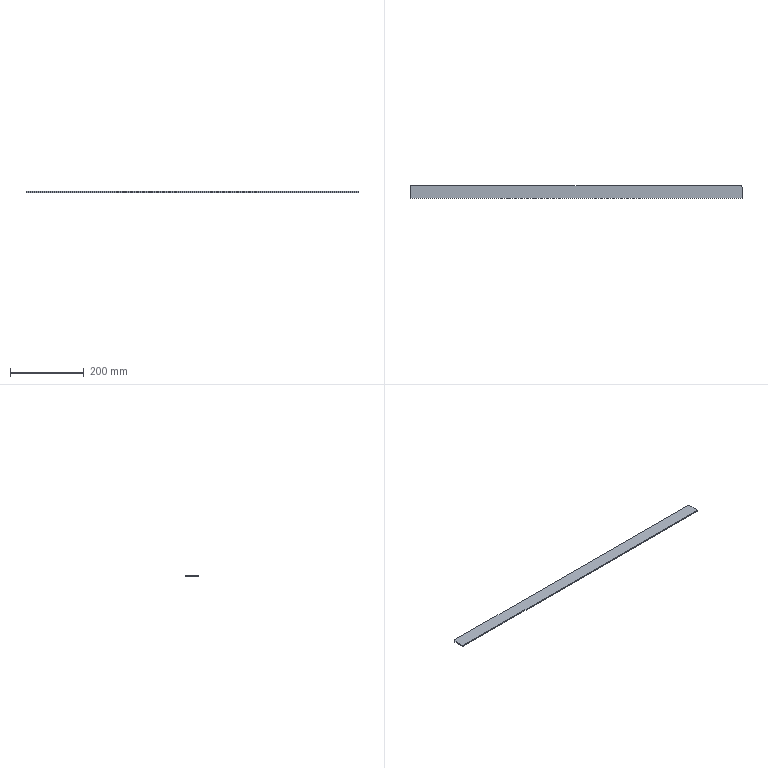Part | SolidWorks | features Extrusion 1, Fillet 1 | 1 solid | 8 faces | box 900 x 35 x 3 mm | volume 94468 mm3 | plane 6 | cylinder 2 | commonest cylinder face diameters 10 x2
STEP:
#1=CARTESIAN_POINT('',(450.,-17.5,0.));
#2=VERTEX_POINT('',#1);
#3=CARTESIAN_POINT('',(450.,12.5,0.));
#4=VERTEX_POINT('',#3);
#5=CARTESIAN_POINT('',(450.,17.5,0.));
#6=DIRECTION('',(0.,1.,0.));
#7=VECTOR('',#6,1000.);
#8=LINE('',#5,#7);
#9=EDGE_CURVE('',#2,#4,#8,.T.);
#10=ORIENTED_EDGE('',*,*,#9,.T.);
#11=CARTESIAN_POINT('',(450.,12.5,3.));
#12=VERTEX_POINT('',#11);
#13=CARTESIAN_POINT('',(450.,12.5,3.));
#14=DIRECTION('',(0.,0.,1.));
#15=VECTOR('',#14,1000.);
#16=LINE('',#13,#15);
#17=EDGE_CURVE('',#4,#12,#16,.T.);
#18=ORIENTED_EDGE('',*,*,#17,.T.);
#19=CARTESIAN_POINT('',(450.,-17.5,3.));
#20=VERTEX_POINT('',#19);
#21=CARTESIAN_POINT('',(450.,17.5,3.));
#22=DIRECTION('',(0.,1.,0.));
#23=VECTOR('',#22,1000.);
#24=LINE('',#21,#23);
#25=EDGE_CURVE('',#20,#12,#24,.T.);
#26=ORIENTED_EDGE('',*,*,#25,.F.);
#27=CARTESIAN_POINT('',(450.,-17.5,3.));
#28=DIRECTION('',(0.,0.,-1.));
#29=VECTOR('',#28,1000.);
#30=LINE('',#27,#29);
#31=EDGE_CURVE('',#20,#2,#30,.T.);
#32=ORIENTED_EDGE('',*,*,#31,.T.);
#33=EDGE_LOOP('',(#10,#18,#26,#32));
#34=FACE_OUTER_BOUND('',#33,.T.);
#35=CARTESIAN_POINT('',(450.,17.5,3.));
#36=DIRECTION('',(-1.,0.,0.));
#37=DIRECTION('',(0.,0.,1.));
#38=AXIS2_PLACEMENT_3D('',#35,#36,#37);
#39=PLANE('',#38);
#40=ADVANCED_FACE('',(#34),#39,.F.);
#41=CARTESIAN_POINT('',(445.,17.5,0.));
#42=VERTEX_POINT('',#41);
#43=CARTESIAN_POINT('',(-445.,17.5,0.));
#44=VERTEX_POINT('',#43);
#45=CARTESIAN_POINT('',(-450.,17.5,0.));
#46=DIRECTION('',(-1.,0.,0.));
#47=VECTOR('',#46,1000.);
#48=LINE('',#45,#47);
#49=EDGE_CURVE('',#42,#44,#48,.T.);
#50=ORIENTED_EDGE('',*,*,#49,.T.);
#51=CARTESIAN_POINT('',(-445.,17.5,3.));
#52=VERTEX_POINT('',#51);
#53=CARTESIAN_POINT('',(-445.,17.5,3.));
#54=DIRECTION('',(0.,0.,1.));
#55=VECTOR('',#54,1000.);
#56=LINE('',#53,#55);
#57=EDGE_CURVE('',#44,#52,#56,.T.);
#58=ORIENTED_EDGE('',*,*,#57,.T.);
#59=CARTESIAN_POINT('',(445.,17.5,3.));
#60=VERTEX_POINT('',#59);
#61=CARTESIAN_POINT('',(-450.,17.5,3.));
#62=DIRECTION('',(-1.,0.,0.));
#63=VECTOR('',#62,1000.);
#64=LINE('',#61,#63);
#65=EDGE_CURVE('',#60,#52,#64,.T.);
#66=ORIENTED_EDGE('',*,*,#65,.F.);
#67=CARTESIAN_POINT('',(445.,17.5,3.));
#68=DIRECTION('',(0.,0.,-1.));
#69=VECTOR('',#68,1000.);
#70=LINE('',#67,#69);
#71=EDGE_CURVE('',#60,#42,#70,.T.);
#72=ORIENTED_EDGE('',*,*,#71,.T.);
#73=EDGE_LOOP('',(#50,#58,#66,#72));
#74=FACE_OUTER_BOUND('',#73,.T.);
#75=CARTESIAN_POINT('',(-450.,17.5,3.));
#76=DIRECTION('',(0.,-1.,0.));
#77=DIRECTION('',(0.,0.,-1.));
#78=AXIS2_PLACEMENT_3D('',#75,#76,#77);
#79=PLANE('',#78);
#80=ADVANCED_FACE('',(#74),#79,.F.);
#81=CARTESIAN_POINT('',(-450.,12.5,3.));
#82=VERTEX_POINT('',#81);
#83=CARTESIAN_POINT('',(-450.,-17.5,3.));
#84=VERTEX_POINT('',#83);
#85=CARTESIAN_POINT('',(-450.,17.5,3.));
#86=DIRECTION('',(0.,-1.,0.));
#87=VECTOR('',#86,1000.);
#88=LINE('',#85,#87);
#89=EDGE_CURVE('',#82,#84,#88,.T.);
#90=ORIENTED_EDGE('',*,*,#89,.F.);
#91=CARTESIAN_POINT('',(-450.,12.5,0.));
#92=VERTEX_POINT('',#91);
#93=CARTESIAN_POINT('',(-450.,12.5,3.));
#94=DIRECTION('',(0.,0.,-1.));
#95=VECTOR('',#94,1000.);
#96=LINE('',#93,#95);
#97=EDGE_CURVE('',#82,#92,#96,.T.);
#98=ORIENTED_EDGE('',*,*,#97,.T.);
#99=CARTESIAN_POINT('',(-450.,-17.5,0.));
#100=VERTEX_POINT('',#99);
#101=CARTESIAN_POINT('',(-450.,17.5,0.));
#102=DIRECTION('',(0.,-1.,0.));
#103=VECTOR('',#102,1000.);
#104=LINE('',#101,#103);
#105=EDGE_CURVE('',#92,#100,#104,.T.);
#106=ORIENTED_EDGE('',*,*,#105,.T.);
#107=CARTESIAN_POINT('',(-450.,-17.5,3.));
#108=DIRECTION('',(0.,0.,-1.));
#109=VECTOR('',#108,1000.);
#110=LINE('',#107,#109);
#111=EDGE_CURVE('',#84,#100,#110,.T.);
#112=ORIENTED_EDGE('',*,*,#111,.F.);
#113=EDGE_LOOP('',(#90,#98,#106,#112));
#114=FACE_OUTER_BOUND('',#113,.T.);
#115=CARTESIAN_POINT('',(-450.,17.5,3.));
#116=DIRECTION('',(1.,0.,0.));
#117=DIRECTION('',(0.,0.,-1.));
#118=AXIS2_PLACEMENT_3D('',#115,#116,#117);
#119=PLANE('',#118);
#120=ADVANCED_FACE('',(#114),#119,.F.);
#121=CARTESIAN_POINT('',(-450.,-17.5,0.));
#122=DIRECTION('',(1.,0.,0.));
#123=VECTOR('',#122,1000.);
#124=LINE('',#121,#123);
#125=EDGE_CURVE('',#100,#2,#124,.T.);
#126=ORIENTED_EDGE('',*,*,#125,.T.);
#127=ORIENTED_EDGE('',*,*,#31,.F.);
#128=CARTESIAN_POINT('',(-450.,-17.5,3.));
#129=DIRECTION('',(1.,0.,0.));
#130=VECTOR('',#129,1000.);
#131=LINE('',#128,#130);
#132=EDGE_CURVE('',#84,#20,#131,.T.);
#133=ORIENTED_EDGE('',*,*,#132,.F.);
#134=ORIENTED_EDGE('',*,*,#111,.T.);
#135=EDGE_LOOP('',(#126,#127,#133,#134));
#136=FACE_OUTER_BOUND('',#135,.T.);
#137=CARTESIAN_POINT('',(-450.,-17.5,3.));
#138=DIRECTION('',(0.,1.,0.));
#139=DIRECTION('',(0.,0.,1.));
#140=AXIS2_PLACEMENT_3D('',#137,#138,#139);
#141=PLANE('',#140);
#142=ADVANCED_FACE('',(#136),#141,.F.);
#143=ORIENTED_EDGE('',*,*,#65,.T.);
#144=CARTESIAN_POINT('',(-445.,12.5,3.));
#145=DIRECTION('',(0.,0.,1.));
#146=DIRECTION('',(1.,0.,0.));
#147=AXIS2_PLACEMENT_3D('',#144,#145,#146);
#148=CIRCLE('',#147,5.);
#149=EDGE_CURVE('',#52,#82,#148,.T.);
#150=ORIENTED_EDGE('',*,*,#149,.T.);
#151=ORIENTED_EDGE('',*,*,#89,.T.);
#152=ORIENTED_EDGE('',*,*,#132,.T.);
#153=ORIENTED_EDGE('',*,*,#25,.T.);
#154=CARTESIAN_POINT('',(445.,12.5,3.));
#155=DIRECTION('',(0.,0.,1.));
#156=DIRECTION('',(1.,0.,0.));
#157=AXIS2_PLACEMENT_3D('',#154,#155,#156);
#158=CIRCLE('',#157,5.);
#159=EDGE_CURVE('',#12,#60,#158,.T.);
#160=ORIENTED_EDGE('',*,*,#159,.T.);
#161=EDGE_LOOP('',(#143,#150,#151,#152,#153,#160));
#162=FACE_OUTER_BOUND('',#161,.T.);
#163=CARTESIAN_POINT('',(0.,0.,3.));
#164=DIRECTION('',(0.,0.,1.));
#165=DIRECTION('',(1.,0.,0.));
#166=AXIS2_PLACEMENT_3D('',#163,#164,#165);
#167=PLANE('',#166);
#168=ADVANCED_FACE('',(#162),#167,.T.);
#169=ORIENTED_EDGE('',*,*,#105,.F.);
#170=CARTESIAN_POINT('',(-445.,12.5,0.));
#171=DIRECTION('',(0.,0.,-1.));
#172=DIRECTION('',(1.,0.,0.));
#173=AXIS2_PLACEMENT_3D('',#170,#171,#172);
#174=CIRCLE('',#173,5.);
#175=EDGE_CURVE('',#92,#44,#174,.T.);
#176=ORIENTED_EDGE('',*,*,#175,.T.);
#177=ORIENTED_EDGE('',*,*,#49,.F.);
#178=CARTESIAN_POINT('',(445.,12.5,0.));
#179=DIRECTION('',(0.,0.,-1.));
#180=DIRECTION('',(1.,0.,0.));
#181=AXIS2_PLACEMENT_3D('',#178,#179,#180);
#182=CIRCLE('',#181,5.);
#183=EDGE_CURVE('',#42,#4,#182,.T.);
#184=ORIENTED_EDGE('',*,*,#183,.T.);
#185=ORIENTED_EDGE('',*,*,#9,.F.);
#186=ORIENTED_EDGE('',*,*,#125,.F.);
#187=EDGE_LOOP('',(#169,#176,#177,#184,#185,#186));
#188=FACE_OUTER_BOUND('',#187,.T.);
#189=CARTESIAN_POINT('',(0.,0.,0.));
#190=DIRECTION('',(0.,0.,1.));
#191=DIRECTION('',(1.,0.,0.));
#192=AXIS2_PLACEMENT_3D('',#189,#190,#191);
#193=PLANE('',#192);
#194=ADVANCED_FACE('',(#188),#193,.F.);
#195=ORIENTED_EDGE('',*,*,#149,.F.);
#196=ORIENTED_EDGE('',*,*,#57,.F.);
#197=ORIENTED_EDGE('',*,*,#175,.F.);
#198=ORIENTED_EDGE('',*,*,#97,.F.);
#199=EDGE_LOOP('',(#195,#196,#197,#198));
#200=FACE_OUTER_BOUND('',#199,.T.);
#201=CARTESIAN_POINT('',(-445.,12.5,3.));
#202=DIRECTION('',(0.,0.,-1.));
#203=DIRECTION('',(-1.,0.,0.));
#204=AXIS2_PLACEMENT_3D('',#201,#202,#203);
#205=CYLINDRICAL_SURFACE('',#204,5.);
#206=ADVANCED_FACE('',(#200),#205,.T.);
#207=ORIENTED_EDGE('',*,*,#159,.F.);
#208=ORIENTED_EDGE('',*,*,#17,.F.);
#209=ORIENTED_EDGE('',*,*,#183,.F.);
#210=ORIENTED_EDGE('',*,*,#71,.F.);
#211=EDGE_LOOP('',(#207,#208,#209,#210));
#212=FACE_OUTER_BOUND('',#211,.T.);
#213=CARTESIAN_POINT('',(445.,12.5,3.));
#214=DIRECTION('',(0.,0.,-1.));
#215=DIRECTION('',(-1.,0.,0.));
#216=AXIS2_PLACEMENT_3D('',#213,#214,#215);
#217=CYLINDRICAL_SURFACE('',#216,5.);
#218=ADVANCED_FACE('',(#212),#217,.T.);
#219=CLOSED_SHELL('',(#40,#80,#120,#142,#168,#194,#206,#218));
#220=MANIFOLD_SOLID_BREP('',#219);
#221=CARTESIAN_POINT('',(0.,0.,0.));
#222=DIRECTION('',(0.,0.,1.));
#223=DIRECTION('',(1.,0.,0.));
#224=AXIS2_PLACEMENT_3D('',#221,#222,#223);
#225=(LENGTH_UNIT()NAMED_UNIT(*)SI_UNIT(.MILLI.,.METRE.));
#226=UNCERTAINTY_MEASURE_WITH_UNIT(LENGTH_MEASURE(0.00001),#225,'','');
#227=(NAMED_UNIT(*)PLANE_ANGLE_UNIT()SI_UNIT($,.RADIAN.));
#228=(NAMED_UNIT(*)SI_UNIT($,.STERADIAN.)SOLID_ANGLE_UNIT());
#229=(GEOMETRIC_REPRESENTATION_CONTEXT(3)GLOBAL_UNCERTAINTY_ASSIGNED_CONTEXT((#226))GLOBAL_UNIT_ASSIGNED_CONTEXT((#225,#227,#228))REPRESENTATION_CONTEXT('',''));
#230=ADVANCED_BREP_SHAPE_REPRESENTATION('',(#220,#224),#229);